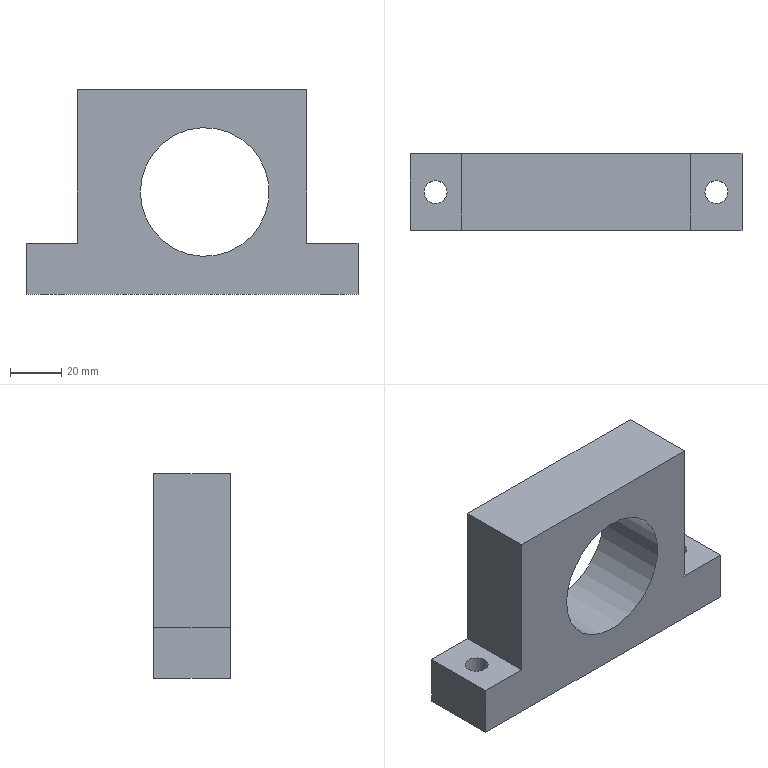Part | NX | features MAIN_BODY 2 | 1 solid | 13 faces | box 130 x 30 x 80 mm | volume 177604 mm3 | plane 10 | cylinder 3 | commonest cylinder face diameters 9 x2 50.4 x1
STEP:
#1=CARTESIAN_POINT('',(-965.,-756.,-415.));
#2=VERTEX_POINT('',#1);
#3=CARTESIAN_POINT('',(-965.,-786.,-415.));
#4=VERTEX_POINT('',#3);
#5=CARTESIAN_POINT('',(-965.,-748.,-415.));
#6=DIRECTION('',(0.,-1.,0.));
#7=VECTOR('',#6,1000.);
#8=LINE('',#5,#7);
#9=EDGE_CURVE('',#2,#4,#8,.T.);
#10=ORIENTED_EDGE('',*,*,#9,.T.);
#11=CARTESIAN_POINT('',(-965.,-786.,-435.));
#12=VERTEX_POINT('',#11);
#13=CARTESIAN_POINT('',(-965.,-786.,-435.));
#14=DIRECTION('',(0.,0.,1.));
#15=VECTOR('',#14,1000.);
#16=LINE('',#13,#15);
#17=EDGE_CURVE('',#12,#4,#16,.T.);
#18=ORIENTED_EDGE('',*,*,#17,.F.);
#19=CARTESIAN_POINT('',(-965.,-756.,-435.));
#20=VERTEX_POINT('',#19);
#21=CARTESIAN_POINT('',(-965.,-756.,-435.));
#22=DIRECTION('',(0.,-1.,0.));
#23=VECTOR('',#22,1000.);
#24=LINE('',#21,#23);
#25=EDGE_CURVE('',#20,#12,#24,.T.);
#26=ORIENTED_EDGE('',*,*,#25,.F.);
#27=CARTESIAN_POINT('',(-965.,-756.,-435.));
#28=DIRECTION('',(0.,0.,1.));
#29=VECTOR('',#28,1000.);
#30=LINE('',#27,#29);
#31=EDGE_CURVE('',#20,#2,#30,.T.);
#32=ORIENTED_EDGE('',*,*,#31,.T.);
#33=EDGE_LOOP('',(#10,#18,#26,#32));
#34=FACE_BOUND('',#33,.T.);
#35=CARTESIAN_POINT('',(-965.,-756.,-435.));
#36=DIRECTION('',(1.,0.,0.));
#37=DIRECTION('',(0.,0.,-1.));
#38=AXIS2_PLACEMENT_3D('',#35,#36,#37);
#39=PLANE('',#38);
#40=ADVANCED_FACE('',(#34),#39,.T.);
#41=CARTESIAN_POINT('',(-1075.,-756.,-355.));
#42=VERTEX_POINT('',#41);
#43=CARTESIAN_POINT('',(-1075.,-786.,-355.));
#44=VERTEX_POINT('',#43);
#45=CARTESIAN_POINT('',(-1075.,-748.,-355.));
#46=DIRECTION('',(0.,-1.,0.));
#47=VECTOR('',#46,1000.);
#48=LINE('',#45,#47);
#49=EDGE_CURVE('',#42,#44,#48,.T.);
#50=ORIENTED_EDGE('',*,*,#49,.T.);
#51=CARTESIAN_POINT('',(-985.,-786.,-355.));
#52=VERTEX_POINT('',#51);
#53=CARTESIAN_POINT('',(-965.,-786.,-355.));
#54=DIRECTION('',(-1.,0.,0.));
#55=VECTOR('',#54,1000.);
#56=LINE('',#53,#55);
#57=EDGE_CURVE('',#52,#44,#56,.T.);
#58=ORIENTED_EDGE('',*,*,#57,.F.);
#59=CARTESIAN_POINT('',(-985.,-756.,-355.));
#60=VERTEX_POINT('',#59);
#61=CARTESIAN_POINT('',(-985.,-748.,-355.));
#62=DIRECTION('',(0.,-1.,0.));
#63=VECTOR('',#62,1000.);
#64=LINE('',#61,#63);
#65=EDGE_CURVE('',#60,#52,#64,.T.);
#66=ORIENTED_EDGE('',*,*,#65,.F.);
#67=CARTESIAN_POINT('',(-965.,-756.,-355.));
#68=DIRECTION('',(-1.,0.,0.));
#69=VECTOR('',#68,1000.);
#70=LINE('',#67,#69);
#71=EDGE_CURVE('',#60,#42,#70,.T.);
#72=ORIENTED_EDGE('',*,*,#71,.T.);
#73=EDGE_LOOP('',(#50,#58,#66,#72));
#74=FACE_BOUND('',#73,.T.);
#75=CARTESIAN_POINT('',(-965.,-756.,-355.));
#76=DIRECTION('',(0.,0.,1.));
#77=DIRECTION('',(0.,1.,0.));
#78=AXIS2_PLACEMENT_3D('',#75,#76,#77);
#79=PLANE('',#78);
#80=ADVANCED_FACE('',(#74),#79,.T.);
#81=CARTESIAN_POINT('',(-1095.,-756.,-415.));
#82=VERTEX_POINT('',#81);
#83=CARTESIAN_POINT('',(-1095.,-786.,-415.));
#84=VERTEX_POINT('',#83);
#85=CARTESIAN_POINT('',(-1095.,-748.,-415.));
#86=DIRECTION('',(0.,-1.,0.));
#87=VECTOR('',#86,1000.);
#88=LINE('',#85,#87);
#89=EDGE_CURVE('',#82,#84,#88,.T.);
#90=ORIENTED_EDGE('',*,*,#89,.F.);
#91=CARTESIAN_POINT('',(-1095.,-756.,-435.));
#92=VERTEX_POINT('',#91);
#93=CARTESIAN_POINT('',(-1095.,-756.,-355.));
#94=DIRECTION('',(0.,0.,-1.));
#95=VECTOR('',#94,1000.);
#96=LINE('',#93,#95);
#97=EDGE_CURVE('',#82,#92,#96,.T.);
#98=ORIENTED_EDGE('',*,*,#97,.T.);
#99=CARTESIAN_POINT('',(-1095.,-786.,-435.));
#100=VERTEX_POINT('',#99);
#101=CARTESIAN_POINT('',(-1095.,-756.,-435.));
#102=DIRECTION('',(0.,-1.,0.));
#103=VECTOR('',#102,1000.);
#104=LINE('',#101,#103);
#105=EDGE_CURVE('',#92,#100,#104,.T.);
#106=ORIENTED_EDGE('',*,*,#105,.T.);
#107=CARTESIAN_POINT('',(-1095.,-786.,-355.));
#108=DIRECTION('',(0.,0.,-1.));
#109=VECTOR('',#108,1000.);
#110=LINE('',#107,#109);
#111=EDGE_CURVE('',#84,#100,#110,.T.);
#112=ORIENTED_EDGE('',*,*,#111,.F.);
#113=EDGE_LOOP('',(#90,#98,#106,#112));
#114=FACE_BOUND('',#113,.T.);
#115=CARTESIAN_POINT('',(-1095.,-756.,-355.));
#116=DIRECTION('',(-1.,0.,0.));
#117=DIRECTION('',(0.,0.,1.));
#118=AXIS2_PLACEMENT_3D('',#115,#116,#117);
#119=PLANE('',#118);
#120=ADVANCED_FACE('',(#114),#119,.T.);
#121=CARTESIAN_POINT('',(-1089.5,-771.,-435.));
#122=VERTEX_POINT('',#121);
#123=CARTESIAN_POINT('',(-1085.,-771.,-435.));
#124=DIRECTION('',(0.,0.,-1.));
#125=DIRECTION('',(-1.,0.,0.));
#126=AXIS2_PLACEMENT_3D('',#123,#124,#125);
#127=CIRCLE('',#126,4.5);
#128=EDGE_CURVE('',#122,#122,#127,.T.);
#129=ORIENTED_EDGE('',*,*,#128,.F.);
#130=EDGE_LOOP('',(#129));
#131=FACE_BOUND('',#130,.T.);
#132=CARTESIAN_POINT('',(-979.5,-771.,-435.));
#133=VERTEX_POINT('',#132);
#134=CARTESIAN_POINT('',(-975.,-771.,-435.));
#135=DIRECTION('',(0.,0.,-1.));
#136=DIRECTION('',(-1.,0.,0.));
#137=AXIS2_PLACEMENT_3D('',#134,#135,#136);
#138=CIRCLE('',#137,4.5);
#139=EDGE_CURVE('',#133,#133,#138,.T.);
#140=ORIENTED_EDGE('',*,*,#139,.F.);
#141=EDGE_LOOP('',(#140));
#142=FACE_BOUND('',#141,.T.);
#143=CARTESIAN_POINT('',(-1095.,-786.,-435.));
#144=DIRECTION('',(1.,0.,0.));
#145=VECTOR('',#144,1000.);
#146=LINE('',#143,#145);
#147=EDGE_CURVE('',#100,#12,#146,.T.);
#148=ORIENTED_EDGE('',*,*,#147,.F.);
#149=ORIENTED_EDGE('',*,*,#105,.F.);
#150=CARTESIAN_POINT('',(-1095.,-756.,-435.));
#151=DIRECTION('',(1.,0.,0.));
#152=VECTOR('',#151,1000.);
#153=LINE('',#150,#152);
#154=EDGE_CURVE('',#92,#20,#153,.T.);
#155=ORIENTED_EDGE('',*,*,#154,.T.);
#156=ORIENTED_EDGE('',*,*,#25,.T.);
#157=EDGE_LOOP('',(#148,#149,#155,#156));
#158=FACE_BOUND('',#157,.T.);
#159=CARTESIAN_POINT('',(-1095.,-756.,-435.));
#160=DIRECTION('',(0.,0.,-1.));
#161=DIRECTION('',(-1.,0.,0.));
#162=AXIS2_PLACEMENT_3D('',#159,#160,#161);
#163=PLANE('',#162);
#164=ADVANCED_FACE('',(#131,#142,#158),#163,.T.);
#165=CARTESIAN_POINT('',(-1050.2,-756.,-395.));
#166=VERTEX_POINT('',#165);
#167=CARTESIAN_POINT('',(-1025.,-756.,-395.));
#168=DIRECTION('',(0.,1.,0.));
#169=DIRECTION('',(-1.,0.,0.));
#170=AXIS2_PLACEMENT_3D('',#167,#168,#169);
#171=CIRCLE('',#170,25.2);
#172=EDGE_CURVE('',#166,#166,#171,.T.);
#173=ORIENTED_EDGE('',*,*,#172,.T.);
#174=EDGE_LOOP('',(#173));
#175=FACE_BOUND('',#174,.T.);
#176=CARTESIAN_POINT('',(-1050.2,-786.,-395.));
#177=VERTEX_POINT('',#176);
#178=CARTESIAN_POINT('',(-1025.,-786.,-395.));
#179=DIRECTION('',(0.,1.,0.));
#180=DIRECTION('',(-1.,0.,0.));
#181=AXIS2_PLACEMENT_3D('',#178,#179,#180);
#182=CIRCLE('',#181,25.2);
#183=EDGE_CURVE('',#177,#177,#182,.T.);
#184=ORIENTED_EDGE('',*,*,#183,.F.);
#185=EDGE_LOOP('',(#184));
#186=FACE_BOUND('',#185,.T.);
#187=CARTESIAN_POINT('',(-1025.,-756.,-395.));
#188=DIRECTION('',(0.,-1.,0.));
#189=DIRECTION('',(1.,0.,0.));
#190=AXIS2_PLACEMENT_3D('',#187,#188,#189);
#191=CYLINDRICAL_SURFACE('',#190,25.2);
#192=ADVANCED_FACE('',(#175,#186),#191,.F.);
#193=CARTESIAN_POINT('',(-1075.,-756.,-415.));
#194=VERTEX_POINT('',#193);
#195=CARTESIAN_POINT('',(-965.,-756.,-415.));
#196=DIRECTION('',(-1.,0.,0.));
#197=VECTOR('',#196,1000.);
#198=LINE('',#195,#197);
#199=EDGE_CURVE('',#194,#82,#198,.T.);
#200=ORIENTED_EDGE('',*,*,#199,.F.);
#201=CARTESIAN_POINT('',(-1075.,-756.,-435.));
#202=DIRECTION('',(0.,0.,-1.));
#203=VECTOR('',#202,1000.);
#204=LINE('',#201,#203);
#205=EDGE_CURVE('',#42,#194,#204,.T.);
#206=ORIENTED_EDGE('',*,*,#205,.F.);
#207=ORIENTED_EDGE('',*,*,#71,.F.);
#208=CARTESIAN_POINT('',(-985.,-756.,-415.));
#209=VERTEX_POINT('',#208);
#210=CARTESIAN_POINT('',(-985.,-756.,-435.));
#211=DIRECTION('',(0.,0.,1.));
#212=VECTOR('',#211,1000.);
#213=LINE('',#210,#212);
#214=EDGE_CURVE('',#209,#60,#213,.T.);
#215=ORIENTED_EDGE('',*,*,#214,.F.);
#216=CARTESIAN_POINT('',(-965.,-756.,-415.));
#217=DIRECTION('',(-1.,0.,0.));
#218=VECTOR('',#217,1000.);
#219=LINE('',#216,#218);
#220=EDGE_CURVE('',#2,#209,#219,.T.);
#221=ORIENTED_EDGE('',*,*,#220,.F.);
#222=ORIENTED_EDGE('',*,*,#31,.F.);
#223=ORIENTED_EDGE('',*,*,#154,.F.);
#224=ORIENTED_EDGE('',*,*,#97,.F.);
#225=EDGE_LOOP('',(#200,#206,#207,#215,#221,#222,#223,#224));
#226=FACE_BOUND('',#225,.T.);
#227=ORIENTED_EDGE('',*,*,#172,.F.);
#228=EDGE_LOOP('',(#227));
#229=FACE_BOUND('',#228,.T.);
#230=CARTESIAN_POINT('',(-965.,-756.,-435.));
#231=DIRECTION('',(0.,1.,0.));
#232=DIRECTION('',(-1.,0.,0.));
#233=AXIS2_PLACEMENT_3D('',#230,#231,#232);
#234=PLANE('',#233);
#235=ADVANCED_FACE('',(#226,#229),#234,.T.);
#236=CARTESIAN_POINT('',(-1075.,-786.,-415.));
#237=VERTEX_POINT('',#236);
#238=CARTESIAN_POINT('',(-1075.,-786.,-435.));
#239=DIRECTION('',(0.,0.,-1.));
#240=VECTOR('',#239,1000.);
#241=LINE('',#238,#240);
#242=EDGE_CURVE('',#44,#237,#241,.T.);
#243=ORIENTED_EDGE('',*,*,#242,.T.);
#244=CARTESIAN_POINT('',(-965.,-786.,-415.));
#245=DIRECTION('',(-1.,0.,0.));
#246=VECTOR('',#245,1000.);
#247=LINE('',#244,#246);
#248=EDGE_CURVE('',#237,#84,#247,.T.);
#249=ORIENTED_EDGE('',*,*,#248,.T.);
#250=ORIENTED_EDGE('',*,*,#111,.T.);
#251=ORIENTED_EDGE('',*,*,#147,.T.);
#252=ORIENTED_EDGE('',*,*,#17,.T.);
#253=CARTESIAN_POINT('',(-985.,-786.,-415.));
#254=VERTEX_POINT('',#253);
#255=CARTESIAN_POINT('',(-965.,-786.,-415.));
#256=DIRECTION('',(-1.,0.,0.));
#257=VECTOR('',#256,1000.);
#258=LINE('',#255,#257);
#259=EDGE_CURVE('',#4,#254,#258,.T.);
#260=ORIENTED_EDGE('',*,*,#259,.T.);
#261=CARTESIAN_POINT('',(-985.,-786.,-435.));
#262=DIRECTION('',(0.,0.,1.));
#263=VECTOR('',#262,1000.);
#264=LINE('',#261,#263);
#265=EDGE_CURVE('',#254,#52,#264,.T.);
#266=ORIENTED_EDGE('',*,*,#265,.T.);
#267=ORIENTED_EDGE('',*,*,#57,.T.);
#268=EDGE_LOOP('',(#243,#249,#250,#251,#252,#260,#266,#267));
#269=FACE_BOUND('',#268,.T.);
#270=ORIENTED_EDGE('',*,*,#183,.T.);
#271=EDGE_LOOP('',(#270));
#272=FACE_BOUND('',#271,.T.);
#273=CARTESIAN_POINT('',(-965.,-786.,-435.));
#274=DIRECTION('',(0.,1.,0.));
#275=DIRECTION('',(-1.,0.,0.));
#276=AXIS2_PLACEMENT_3D('',#273,#274,#275);
#277=PLANE('',#276);
#278=ADVANCED_FACE('',(#269,#272),#277,.F.);
#279=ORIENTED_EDGE('',*,*,#214,.T.);
#280=ORIENTED_EDGE('',*,*,#65,.T.);
#281=ORIENTED_EDGE('',*,*,#265,.F.);
#282=CARTESIAN_POINT('',(-985.,-748.,-415.));
#283=DIRECTION('',(0.,-1.,0.));
#284=VECTOR('',#283,1000.);
#285=LINE('',#282,#284);
#286=EDGE_CURVE('',#209,#254,#285,.T.);
#287=ORIENTED_EDGE('',*,*,#286,.F.);
#288=EDGE_LOOP('',(#279,#280,#281,#287));
#289=FACE_BOUND('',#288,.T.);
#290=CARTESIAN_POINT('',(-985.,-748.,-355.));
#291=DIRECTION('',(-1.,0.,0.));
#292=DIRECTION('',(0.,0.,1.));
#293=AXIS2_PLACEMENT_3D('',#290,#291,#292);
#294=PLANE('',#293);
#295=ADVANCED_FACE('',(#289),#294,.F.);
#296=CARTESIAN_POINT('',(-979.5,-771.,-415.));
#297=VERTEX_POINT('',#296);
#298=CARTESIAN_POINT('',(-975.,-771.,-415.));
#299=DIRECTION('',(0.,0.,-1.));
#300=DIRECTION('',(-1.,0.,0.));
#301=AXIS2_PLACEMENT_3D('',#298,#299,#300);
#302=CIRCLE('',#301,4.5);
#303=EDGE_CURVE('',#297,#297,#302,.T.);
#304=ORIENTED_EDGE('',*,*,#303,.T.);
#305=EDGE_LOOP('',(#304));
#306=FACE_BOUND('',#305,.T.);
#307=ORIENTED_EDGE('',*,*,#220,.T.);
#308=ORIENTED_EDGE('',*,*,#286,.T.);
#309=ORIENTED_EDGE('',*,*,#259,.F.);
#310=ORIENTED_EDGE('',*,*,#9,.F.);
#311=EDGE_LOOP('',(#307,#308,#309,#310));
#312=FACE_BOUND('',#311,.T.);
#313=CARTESIAN_POINT('',(-985.,-748.,-415.));
#314=DIRECTION('',(0.,0.,-1.));
#315=DIRECTION('',(-1.,0.,0.));
#316=AXIS2_PLACEMENT_3D('',#313,#314,#315);
#317=PLANE('',#316);
#318=ADVANCED_FACE('',(#306,#312),#317,.F.);
#319=CARTESIAN_POINT('',(-1089.5,-771.,-415.));
#320=VERTEX_POINT('',#319);
#321=CARTESIAN_POINT('',(-1085.,-771.,-415.));
#322=DIRECTION('',(0.,0.,-1.));
#323=DIRECTION('',(-1.,0.,0.));
#324=AXIS2_PLACEMENT_3D('',#321,#322,#323);
#325=CIRCLE('',#324,4.5);
#326=EDGE_CURVE('',#320,#320,#325,.T.);
#327=ORIENTED_EDGE('',*,*,#326,.T.);
#328=EDGE_LOOP('',(#327));
#329=FACE_BOUND('',#328,.T.);
#330=ORIENTED_EDGE('',*,*,#199,.T.);
#331=ORIENTED_EDGE('',*,*,#89,.T.);
#332=ORIENTED_EDGE('',*,*,#248,.F.);
#333=CARTESIAN_POINT('',(-1075.,-748.,-415.));
#334=DIRECTION('',(0.,-1.,0.));
#335=VECTOR('',#334,1000.);
#336=LINE('',#333,#335);
#337=EDGE_CURVE('',#194,#237,#336,.T.);
#338=ORIENTED_EDGE('',*,*,#337,.F.);
#339=EDGE_LOOP('',(#330,#331,#332,#338));
#340=FACE_BOUND('',#339,.T.);
#341=CARTESIAN_POINT('',(-1095.,-748.,-415.));
#342=DIRECTION('',(0.,0.,-1.));
#343=DIRECTION('',(-1.,0.,0.));
#344=AXIS2_PLACEMENT_3D('',#341,#342,#343);
#345=PLANE('',#344);
#346=ADVANCED_FACE('',(#329,#340),#345,.F.);
#347=ORIENTED_EDGE('',*,*,#205,.T.);
#348=ORIENTED_EDGE('',*,*,#337,.T.);
#349=ORIENTED_EDGE('',*,*,#242,.F.);
#350=ORIENTED_EDGE('',*,*,#49,.F.);
#351=EDGE_LOOP('',(#347,#348,#349,#350));
#352=FACE_BOUND('',#351,.T.);
#353=CARTESIAN_POINT('',(-1075.,-748.,-415.));
#354=DIRECTION('',(1.,0.,0.));
#355=DIRECTION('',(0.,0.,-1.));
#356=AXIS2_PLACEMENT_3D('',#353,#354,#355);
#357=PLANE('',#356);
#358=ADVANCED_FACE('',(#352),#357,.F.);
#359=ORIENTED_EDGE('',*,*,#139,.T.);
#360=EDGE_LOOP('',(#359));
#361=FACE_BOUND('',#360,.T.);
#362=ORIENTED_EDGE('',*,*,#303,.F.);
#363=EDGE_LOOP('',(#362));
#364=FACE_BOUND('',#363,.T.);
#365=CARTESIAN_POINT('',(-975.,-771.,-445.));
#366=DIRECTION('',(0.,0.,1.));
#367=DIRECTION('',(0.,1.,0.));
#368=AXIS2_PLACEMENT_3D('',#365,#366,#367);
#369=CYLINDRICAL_SURFACE('',#368,4.5);
#370=ADVANCED_FACE('',(#361,#364),#369,.F.);
#371=ORIENTED_EDGE('',*,*,#128,.T.);
#372=EDGE_LOOP('',(#371));
#373=FACE_BOUND('',#372,.T.);
#374=ORIENTED_EDGE('',*,*,#326,.F.);
#375=EDGE_LOOP('',(#374));
#376=FACE_BOUND('',#375,.T.);
#377=CARTESIAN_POINT('',(-1085.,-771.,-445.));
#378=DIRECTION('',(0.,0.,1.));
#379=DIRECTION('',(0.,1.,0.));
#380=AXIS2_PLACEMENT_3D('',#377,#378,#379);
#381=CYLINDRICAL_SURFACE('',#380,4.5);
#382=ADVANCED_FACE('',(#373,#376),#381,.F.);
#383=CLOSED_SHELL('',(#40,#80,#120,#164,#192,#235,#278,#295,#318,#346,#358,#370,#382));
#384=MANIFOLD_SOLID_BREP('',#383);
#385=(LENGTH_UNIT()NAMED_UNIT(*)SI_UNIT(.MILLI.,.METRE.));
#386=UNCERTAINTY_MEASURE_WITH_UNIT(LENGTH_MEASURE(0.00001),#385,'','');
#387=(NAMED_UNIT(*)PLANE_ANGLE_UNIT()SI_UNIT($,.RADIAN.));
#388=(NAMED_UNIT(*)SI_UNIT($,.STERADIAN.)SOLID_ANGLE_UNIT());
#389=(GEOMETRIC_REPRESENTATION_CONTEXT(3)GLOBAL_UNCERTAINTY_ASSIGNED_CONTEXT((#386))GLOBAL_UNIT_ASSIGNED_CONTEXT((#385,#387,#388))REPRESENTATION_CONTEXT('',''));
#390=ADVANCED_BREP_SHAPE_REPRESENTATION('',(#384),#389);